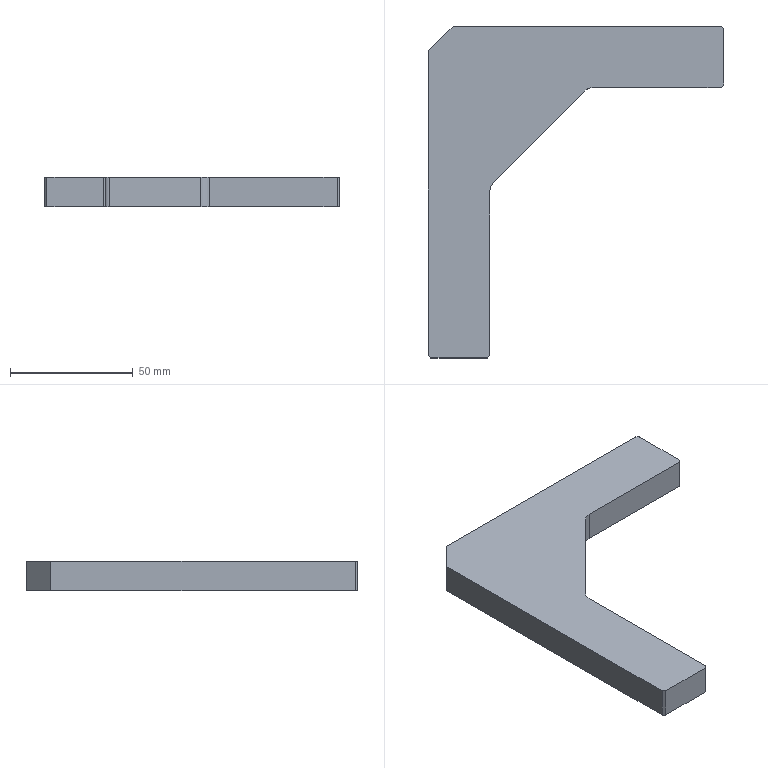Part | SolidWorks | features BaseBody 1 | 1 solid | 16 faces | box 120 x 135 x 12 mm | volume 77989 mm3 | plane 14 | cylinder 2 | commonest cylinder face diameters 10 x2
STEP:
#1=CARTESIAN_POINT('',(120.,-1.,12.));
#2=VERTEX_POINT('',#1);
#3=CARTESIAN_POINT('',(119.,0.,12.));
#4=VERTEX_POINT('',#3);
#5=CARTESIAN_POINT('',(119.,0.,12.));
#6=DIRECTION('',(-0.7071,0.7071,0.));
#7=VECTOR('',#6,1000.);
#8=LINE('',#5,#7);
#9=EDGE_CURVE('',#2,#4,#8,.T.);
#10=ORIENTED_EDGE('',*,*,#9,.F.);
#11=CARTESIAN_POINT('',(120.,-1.,0.));
#12=VERTEX_POINT('',#11);
#13=CARTESIAN_POINT('',(120.,-1.,12.));
#14=DIRECTION('',(0.,0.,1.));
#15=VECTOR('',#14,1000.);
#16=LINE('',#13,#15);
#17=EDGE_CURVE('',#12,#2,#16,.T.);
#18=ORIENTED_EDGE('',*,*,#17,.F.);
#19=CARTESIAN_POINT('',(119.,0.,0.));
#20=VERTEX_POINT('',#19);
#21=CARTESIAN_POINT('',(59.5,59.5,0.));
#22=DIRECTION('',(0.7071,-0.7071,0.));
#23=VECTOR('',#22,1000.);
#24=LINE('',#21,#23);
#25=EDGE_CURVE('',#20,#12,#24,.T.);
#26=ORIENTED_EDGE('',*,*,#25,.F.);
#27=CARTESIAN_POINT('',(119.,0.,12.));
#28=DIRECTION('',(0.,0.,-1.));
#29=VECTOR('',#28,1000.);
#30=LINE('',#27,#29);
#31=EDGE_CURVE('',#4,#20,#30,.T.);
#32=ORIENTED_EDGE('',*,*,#31,.F.);
#33=EDGE_LOOP('',(#10,#18,#26,#32));
#34=FACE_OUTER_BOUND('',#33,.T.);
#35=CARTESIAN_POINT('',(119.,0.,12.));
#36=DIRECTION('',(-0.7071,-0.7071,0.));
#37=DIRECTION('',(-0.7071,0.7071,0.));
#38=AXIS2_PLACEMENT_3D('',#35,#36,#37);
#39=PLANE('',#38);
#40=ADVANCED_FACE('',(#34),#39,.F.);
#41=CARTESIAN_POINT('',(119.,-25.,12.));
#42=VERTEX_POINT('',#41);
#43=CARTESIAN_POINT('',(120.,-24.,12.));
#44=VERTEX_POINT('',#43);
#45=CARTESIAN_POINT('',(120.,-24.,12.));
#46=DIRECTION('',(0.7071,0.7071,0.));
#47=VECTOR('',#46,1000.);
#48=LINE('',#45,#47);
#49=EDGE_CURVE('',#42,#44,#48,.T.);
#50=ORIENTED_EDGE('',*,*,#49,.F.);
#51=CARTESIAN_POINT('',(119.,-25.,0.));
#52=VERTEX_POINT('',#51);
#53=CARTESIAN_POINT('',(119.,-25.,12.));
#54=DIRECTION('',(0.,0.,1.));
#55=VECTOR('',#54,1000.);
#56=LINE('',#53,#55);
#57=EDGE_CURVE('',#52,#42,#56,.T.);
#58=ORIENTED_EDGE('',*,*,#57,.F.);
#59=CARTESIAN_POINT('',(120.,-24.,0.));
#60=VERTEX_POINT('',#59);
#61=CARTESIAN_POINT('',(72.,-72.,0.));
#62=DIRECTION('',(-0.7071,-0.7071,0.));
#63=VECTOR('',#62,1000.);
#64=LINE('',#61,#63);
#65=EDGE_CURVE('',#60,#52,#64,.T.);
#66=ORIENTED_EDGE('',*,*,#65,.F.);
#67=CARTESIAN_POINT('',(120.,-24.,12.));
#68=DIRECTION('',(0.,0.,-1.));
#69=VECTOR('',#68,1000.);
#70=LINE('',#67,#69);
#71=EDGE_CURVE('',#44,#60,#70,.T.);
#72=ORIENTED_EDGE('',*,*,#71,.F.);
#73=EDGE_LOOP('',(#50,#58,#66,#72));
#74=FACE_OUTER_BOUND('',#73,.T.);
#75=CARTESIAN_POINT('',(120.,-24.,12.));
#76=DIRECTION('',(-0.7071,0.7071,0.));
#77=DIRECTION('',(0.,0.,1.));
#78=AXIS2_PLACEMENT_3D('',#75,#76,#77);
#79=PLANE('',#78);
#80=ADVANCED_FACE('',(#74),#79,.F.);
#81=CARTESIAN_POINT('',(24.,-135.,12.));
#82=VERTEX_POINT('',#81);
#83=CARTESIAN_POINT('',(25.,-134.,12.));
#84=VERTEX_POINT('',#83);
#85=CARTESIAN_POINT('',(25.,-134.,12.));
#86=DIRECTION('',(0.7071,0.7071,0.));
#87=VECTOR('',#86,1000.);
#88=LINE('',#85,#87);
#89=EDGE_CURVE('',#82,#84,#88,.T.);
#90=ORIENTED_EDGE('',*,*,#89,.F.);
#91=CARTESIAN_POINT('',(24.,-135.,0.));
#92=VERTEX_POINT('',#91);
#93=CARTESIAN_POINT('',(24.,-135.,12.));
#94=DIRECTION('',(0.,0.,1.));
#95=VECTOR('',#94,1000.);
#96=LINE('',#93,#95);
#97=EDGE_CURVE('',#92,#82,#96,.T.);
#98=ORIENTED_EDGE('',*,*,#97,.F.);
#99=CARTESIAN_POINT('',(25.,-134.,0.));
#100=VERTEX_POINT('',#99);
#101=CARTESIAN_POINT('',(79.5,-79.5,0.));
#102=DIRECTION('',(-0.7071,-0.7071,0.));
#103=VECTOR('',#102,1000.);
#104=LINE('',#101,#103);
#105=EDGE_CURVE('',#100,#92,#104,.T.);
#106=ORIENTED_EDGE('',*,*,#105,.F.);
#107=CARTESIAN_POINT('',(25.,-134.,12.));
#108=DIRECTION('',(0.,0.,-1.));
#109=VECTOR('',#108,1000.);
#110=LINE('',#107,#109);
#111=EDGE_CURVE('',#84,#100,#110,.T.);
#112=ORIENTED_EDGE('',*,*,#111,.F.);
#113=EDGE_LOOP('',(#90,#98,#106,#112));
#114=FACE_OUTER_BOUND('',#113,.T.);
#115=CARTESIAN_POINT('',(25.,-134.,12.));
#116=DIRECTION('',(-0.7071,0.7071,0.));
#117=DIRECTION('',(0.,0.,1.));
#118=AXIS2_PLACEMENT_3D('',#115,#116,#117);
#119=PLANE('',#118);
#120=ADVANCED_FACE('',(#114),#119,.F.);
#121=CARTESIAN_POINT('',(0.,-134.,12.));
#122=VERTEX_POINT('',#121);
#123=CARTESIAN_POINT('',(1.,-135.,12.));
#124=VERTEX_POINT('',#123);
#125=CARTESIAN_POINT('',(1.,-135.,12.));
#126=DIRECTION('',(0.7071,-0.7071,0.));
#127=VECTOR('',#126,1000.);
#128=LINE('',#125,#127);
#129=EDGE_CURVE('',#122,#124,#128,.T.);
#130=ORIENTED_EDGE('',*,*,#129,.F.);
#131=CARTESIAN_POINT('',(0.,-134.,0.));
#132=VERTEX_POINT('',#131);
#133=CARTESIAN_POINT('',(0.,-134.,12.));
#134=DIRECTION('',(0.,0.,1.));
#135=VECTOR('',#134,1000.);
#136=LINE('',#133,#135);
#137=EDGE_CURVE('',#132,#122,#136,.T.);
#138=ORIENTED_EDGE('',*,*,#137,.F.);
#139=CARTESIAN_POINT('',(1.,-135.,0.));
#140=VERTEX_POINT('',#139);
#141=CARTESIAN_POINT('',(-67.,-67.,0.));
#142=DIRECTION('',(-0.7071,0.7071,0.));
#143=VECTOR('',#142,1000.);
#144=LINE('',#141,#143);
#145=EDGE_CURVE('',#140,#132,#144,.T.);
#146=ORIENTED_EDGE('',*,*,#145,.F.);
#147=CARTESIAN_POINT('',(1.,-135.,12.));
#148=DIRECTION('',(0.,0.,-1.));
#149=VECTOR('',#148,1000.);
#150=LINE('',#147,#149);
#151=EDGE_CURVE('',#124,#140,#150,.T.);
#152=ORIENTED_EDGE('',*,*,#151,.F.);
#153=EDGE_LOOP('',(#130,#138,#146,#152));
#154=FACE_OUTER_BOUND('',#153,.T.);
#155=CARTESIAN_POINT('',(1.,-135.,12.));
#156=DIRECTION('',(0.7071,0.7071,0.));
#157=DIRECTION('',(0.,0.,-1.));
#158=AXIS2_PLACEMENT_3D('',#155,#156,#157);
#159=PLANE('',#158);
#160=ADVANCED_FACE('',(#154),#159,.F.);
#161=CARTESIAN_POINT('',(25.,-67.071,12.));
#162=VERTEX_POINT('',#161);
#163=CARTESIAN_POINT('',(26.464,-63.536,12.));
#164=VERTEX_POINT('',#163);
#165=CARTESIAN_POINT('',(30.,-67.071,12.));
#166=DIRECTION('',(0.,0.,-1.));
#167=DIRECTION('',(-1.,0.,0.));
#168=AXIS2_PLACEMENT_3D('',#165,#166,#167);
#169=CIRCLE('',#168,5.);
#170=EDGE_CURVE('',#162,#164,#169,.T.);
#171=ORIENTED_EDGE('',*,*,#170,.F.);
#172=CARTESIAN_POINT('',(25.,-67.071,0.));
#173=VERTEX_POINT('',#172);
#174=CARTESIAN_POINT('',(25.,-67.071,12.));
#175=DIRECTION('',(0.,0.,1.));
#176=VECTOR('',#175,1000.);
#177=LINE('',#174,#176);
#178=EDGE_CURVE('',#173,#162,#177,.T.);
#179=ORIENTED_EDGE('',*,*,#178,.F.);
#180=CARTESIAN_POINT('',(26.464,-63.536,0.));
#181=VERTEX_POINT('',#180);
#182=CARTESIAN_POINT('',(30.,-67.071,0.));
#183=DIRECTION('',(0.,0.,1.));
#184=DIRECTION('',(-1.,0.,0.));
#185=AXIS2_PLACEMENT_3D('',#182,#183,#184);
#186=CIRCLE('',#185,5.);
#187=EDGE_CURVE('',#181,#173,#186,.T.);
#188=ORIENTED_EDGE('',*,*,#187,.F.);
#189=CARTESIAN_POINT('',(26.464,-63.536,0.));
#190=DIRECTION('',(0.,0.,-1.));
#191=VECTOR('',#190,1000.);
#192=LINE('',#189,#191);
#193=EDGE_CURVE('',#164,#181,#192,.T.);
#194=ORIENTED_EDGE('',*,*,#193,.F.);
#195=EDGE_LOOP('',(#171,#179,#188,#194));
#196=FACE_OUTER_BOUND('',#195,.T.);
#197=CARTESIAN_POINT('',(30.,-67.071,12.));
#198=DIRECTION('',(0.,0.,1.));
#199=DIRECTION('',(1.,0.,0.));
#200=AXIS2_PLACEMENT_3D('',#197,#198,#199);
#201=CYLINDRICAL_SURFACE('',#200,5.);
#202=ADVANCED_FACE('',(#196),#201,.F.);
#203=CARTESIAN_POINT('',(63.536,-26.464,12.));
#204=VERTEX_POINT('',#203);
#205=CARTESIAN_POINT('',(67.071,-25.,12.));
#206=VERTEX_POINT('',#205);
#207=CARTESIAN_POINT('',(67.071,-30.,12.));
#208=DIRECTION('',(0.,0.,-1.));
#209=DIRECTION('',(-1.,0.,0.));
#210=AXIS2_PLACEMENT_3D('',#207,#208,#209);
#211=CIRCLE('',#210,5.);
#212=EDGE_CURVE('',#204,#206,#211,.T.);
#213=ORIENTED_EDGE('',*,*,#212,.F.);
#214=CARTESIAN_POINT('',(63.536,-26.464,0.));
#215=VERTEX_POINT('',#214);
#216=CARTESIAN_POINT('',(63.536,-26.464,12.));
#217=DIRECTION('',(0.,0.,1.));
#218=VECTOR('',#217,1000.);
#219=LINE('',#216,#218);
#220=EDGE_CURVE('',#215,#204,#219,.T.);
#221=ORIENTED_EDGE('',*,*,#220,.F.);
#222=CARTESIAN_POINT('',(67.071,-25.,0.));
#223=VERTEX_POINT('',#222);
#224=CARTESIAN_POINT('',(67.071,-30.,0.));
#225=DIRECTION('',(0.,0.,1.));
#226=DIRECTION('',(-1.,0.,0.));
#227=AXIS2_PLACEMENT_3D('',#224,#225,#226);
#228=CIRCLE('',#227,5.);
#229=EDGE_CURVE('',#223,#215,#228,.T.);
#230=ORIENTED_EDGE('',*,*,#229,.F.);
#231=CARTESIAN_POINT('',(67.071,-25.,0.));
#232=DIRECTION('',(0.,0.,-1.));
#233=VECTOR('',#232,1000.);
#234=LINE('',#231,#233);
#235=EDGE_CURVE('',#206,#223,#234,.T.);
#236=ORIENTED_EDGE('',*,*,#235,.F.);
#237=EDGE_LOOP('',(#213,#221,#230,#236));
#238=FACE_OUTER_BOUND('',#237,.T.);
#239=CARTESIAN_POINT('',(67.071,-30.,12.));
#240=DIRECTION('',(0.,0.,1.));
#241=DIRECTION('',(1.,0.,0.));
#242=AXIS2_PLACEMENT_3D('',#239,#240,#241);
#243=CYLINDRICAL_SURFACE('',#242,5.);
#244=ADVANCED_FACE('',(#238),#243,.F.);
#245=CARTESIAN_POINT('',(10.,0.,12.));
#246=VERTEX_POINT('',#245);
#247=CARTESIAN_POINT('',(0.,-10.,12.));
#248=VERTEX_POINT('',#247);
#249=CARTESIAN_POINT('',(0.,-10.,12.));
#250=DIRECTION('',(-0.7071,-0.7071,0.));
#251=VECTOR('',#250,1000.);
#252=LINE('',#249,#251);
#253=EDGE_CURVE('',#246,#248,#252,.T.);
#254=ORIENTED_EDGE('',*,*,#253,.F.);
#255=CARTESIAN_POINT('',(10.,0.,0.));
#256=VERTEX_POINT('',#255);
#257=CARTESIAN_POINT('',(10.,0.,12.));
#258=DIRECTION('',(0.,0.,1.));
#259=VECTOR('',#258,1000.);
#260=LINE('',#257,#259);
#261=EDGE_CURVE('',#256,#246,#260,.T.);
#262=ORIENTED_EDGE('',*,*,#261,.F.);
#263=CARTESIAN_POINT('',(0.,-10.,0.));
#264=VERTEX_POINT('',#263);
#265=CARTESIAN_POINT('',(5.,-5.,0.));
#266=DIRECTION('',(0.7071,0.7071,0.));
#267=VECTOR('',#266,1000.);
#268=LINE('',#265,#267);
#269=EDGE_CURVE('',#264,#256,#268,.T.);
#270=ORIENTED_EDGE('',*,*,#269,.F.);
#271=CARTESIAN_POINT('',(0.,-10.,12.));
#272=DIRECTION('',(0.,0.,-1.));
#273=VECTOR('',#272,1000.);
#274=LINE('',#271,#273);
#275=EDGE_CURVE('',#248,#264,#274,.T.);
#276=ORIENTED_EDGE('',*,*,#275,.F.);
#277=EDGE_LOOP('',(#254,#262,#270,#276));
#278=FACE_OUTER_BOUND('',#277,.T.);
#279=CARTESIAN_POINT('',(0.,-10.,12.));
#280=DIRECTION('',(0.7071,-0.7071,0.));
#281=DIRECTION('',(0.,0.,-1.));
#282=AXIS2_PLACEMENT_3D('',#279,#280,#281);
#283=PLANE('',#282);
#284=ADVANCED_FACE('',(#278),#283,.F.);
#285=CARTESIAN_POINT('',(25.,-135.,0.));
#286=DIRECTION('',(1.,0.,0.));
#287=VECTOR('',#286,1000.);
#288=LINE('',#285,#287);
#289=EDGE_CURVE('',#140,#92,#288,.T.);
#290=ORIENTED_EDGE('',*,*,#289,.F.);
#291=ORIENTED_EDGE('',*,*,#145,.T.);
#292=CARTESIAN_POINT('',(0.,-135.,0.));
#293=DIRECTION('',(0.,-1.,0.));
#294=VECTOR('',#293,1000.);
#295=LINE('',#292,#294);
#296=EDGE_CURVE('',#264,#132,#295,.T.);
#297=ORIENTED_EDGE('',*,*,#296,.F.);
#298=ORIENTED_EDGE('',*,*,#269,.T.);
#299=CARTESIAN_POINT('',(0.,0.,0.));
#300=DIRECTION('',(-1.,0.,0.));
#301=VECTOR('',#300,1000.);
#302=LINE('',#299,#301);
#303=EDGE_CURVE('',#20,#256,#302,.T.);
#304=ORIENTED_EDGE('',*,*,#303,.F.);
#305=ORIENTED_EDGE('',*,*,#25,.T.);
#306=CARTESIAN_POINT('',(120.,0.,0.));
#307=DIRECTION('',(0.,1.,0.));
#308=VECTOR('',#307,1000.);
#309=LINE('',#306,#308);
#310=EDGE_CURVE('',#60,#12,#309,.T.);
#311=ORIENTED_EDGE('',*,*,#310,.F.);
#312=ORIENTED_EDGE('',*,*,#65,.T.);
#313=CARTESIAN_POINT('',(120.,-25.,0.));
#314=DIRECTION('',(1.,0.,0.));
#315=VECTOR('',#314,1000.);
#316=LINE('',#313,#315);
#317=EDGE_CURVE('',#223,#52,#316,.T.);
#318=ORIENTED_EDGE('',*,*,#317,.F.);
#319=ORIENTED_EDGE('',*,*,#229,.T.);
#320=CARTESIAN_POINT('',(65.,-25.,0.));
#321=DIRECTION('',(0.7071,0.7071,0.));
#322=VECTOR('',#321,1000.);
#323=LINE('',#320,#322);
#324=EDGE_CURVE('',#181,#215,#323,.T.);
#325=ORIENTED_EDGE('',*,*,#324,.F.);
#326=ORIENTED_EDGE('',*,*,#187,.T.);
#327=CARTESIAN_POINT('',(25.,-65.,0.));
#328=DIRECTION('',(0.,1.,0.));
#329=VECTOR('',#328,1000.);
#330=LINE('',#327,#329);
#331=EDGE_CURVE('',#100,#173,#330,.T.);
#332=ORIENTED_EDGE('',*,*,#331,.F.);
#333=ORIENTED_EDGE('',*,*,#105,.T.);
#334=EDGE_LOOP('',(#290,#291,#297,#298,#304,#305,#311,#312,#318,#319,#325,#326,#332,#333));
#335=FACE_OUTER_BOUND('',#334,.T.);
#336=CARTESIAN_POINT('',(0.,0.,0.));
#337=DIRECTION('',(0.,0.,-1.));
#338=DIRECTION('',(0.,-1.,0.));
#339=AXIS2_PLACEMENT_3D('',#336,#337,#338);
#340=PLANE('',#339);
#341=ADVANCED_FACE('',(#335),#340,.T.);
#342=CARTESIAN_POINT('',(0.,-135.,12.));
#343=DIRECTION('',(0.,-1.,0.));
#344=VECTOR('',#343,1000.);
#345=LINE('',#342,#344);
#346=EDGE_CURVE('',#248,#122,#345,.T.);
#347=ORIENTED_EDGE('',*,*,#346,.T.);
#348=ORIENTED_EDGE('',*,*,#129,.T.);
#349=CARTESIAN_POINT('',(25.,-135.,12.));
#350=DIRECTION('',(1.,0.,0.));
#351=VECTOR('',#350,1000.);
#352=LINE('',#349,#351);
#353=EDGE_CURVE('',#124,#82,#352,.T.);
#354=ORIENTED_EDGE('',*,*,#353,.T.);
#355=ORIENTED_EDGE('',*,*,#89,.T.);
#356=CARTESIAN_POINT('',(25.,-65.,12.));
#357=DIRECTION('',(0.,1.,0.));
#358=VECTOR('',#357,1000.);
#359=LINE('',#356,#358);
#360=EDGE_CURVE('',#84,#162,#359,.T.);
#361=ORIENTED_EDGE('',*,*,#360,.T.);
#362=ORIENTED_EDGE('',*,*,#170,.T.);
#363=CARTESIAN_POINT('',(65.,-25.,12.));
#364=DIRECTION('',(0.7071,0.7071,0.));
#365=VECTOR('',#364,1000.);
#366=LINE('',#363,#365);
#367=EDGE_CURVE('',#164,#204,#366,.T.);
#368=ORIENTED_EDGE('',*,*,#367,.T.);
#369=ORIENTED_EDGE('',*,*,#212,.T.);
#370=CARTESIAN_POINT('',(120.,-25.,12.));
#371=DIRECTION('',(1.,0.,0.));
#372=VECTOR('',#371,1000.);
#373=LINE('',#370,#372);
#374=EDGE_CURVE('',#206,#42,#373,.T.);
#375=ORIENTED_EDGE('',*,*,#374,.T.);
#376=ORIENTED_EDGE('',*,*,#49,.T.);
#377=CARTESIAN_POINT('',(120.,0.,12.));
#378=DIRECTION('',(0.,1.,0.));
#379=VECTOR('',#378,1000.);
#380=LINE('',#377,#379);
#381=EDGE_CURVE('',#44,#2,#380,.T.);
#382=ORIENTED_EDGE('',*,*,#381,.T.);
#383=ORIENTED_EDGE('',*,*,#9,.T.);
#384=CARTESIAN_POINT('',(0.,0.,12.));
#385=DIRECTION('',(-1.,0.,0.));
#386=VECTOR('',#385,1000.);
#387=LINE('',#384,#386);
#388=EDGE_CURVE('',#4,#246,#387,.T.);
#389=ORIENTED_EDGE('',*,*,#388,.T.);
#390=ORIENTED_EDGE('',*,*,#253,.T.);
#391=EDGE_LOOP('',(#347,#348,#354,#355,#361,#362,#368,#369,#375,#376,#382,#383,#389,#390));
#392=FACE_OUTER_BOUND('',#391,.T.);
#393=CARTESIAN_POINT('',(0.,0.,12.));
#394=DIRECTION('',(0.,0.,-1.));
#395=DIRECTION('',(0.,-1.,0.));
#396=AXIS2_PLACEMENT_3D('',#393,#394,#395);
#397=PLANE('',#396);
#398=ADVANCED_FACE('',(#392),#397,.F.);
#399=ORIENTED_EDGE('',*,*,#388,.F.);
#400=ORIENTED_EDGE('',*,*,#31,.T.);
#401=ORIENTED_EDGE('',*,*,#303,.T.);
#402=ORIENTED_EDGE('',*,*,#261,.T.);
#403=EDGE_LOOP('',(#399,#400,#401,#402));
#404=FACE_OUTER_BOUND('',#403,.T.);
#405=CARTESIAN_POINT('',(0.,0.,12.));
#406=DIRECTION('',(0.,-1.,0.));
#407=DIRECTION('',(0.,0.,-1.));
#408=AXIS2_PLACEMENT_3D('',#405,#406,#407);
#409=PLANE('',#408);
#410=ADVANCED_FACE('',(#404),#409,.F.);
#411=ORIENTED_EDGE('',*,*,#381,.F.);
#412=ORIENTED_EDGE('',*,*,#71,.T.);
#413=ORIENTED_EDGE('',*,*,#310,.T.);
#414=ORIENTED_EDGE('',*,*,#17,.T.);
#415=EDGE_LOOP('',(#411,#412,#413,#414));
#416=FACE_OUTER_BOUND('',#415,.T.);
#417=CARTESIAN_POINT('',(120.,0.,12.));
#418=DIRECTION('',(-1.,0.,0.));
#419=DIRECTION('',(0.,0.,1.));
#420=AXIS2_PLACEMENT_3D('',#417,#418,#419);
#421=PLANE('',#420);
#422=ADVANCED_FACE('',(#416),#421,.F.);
#423=ORIENTED_EDGE('',*,*,#317,.T.);
#424=ORIENTED_EDGE('',*,*,#57,.T.);
#425=ORIENTED_EDGE('',*,*,#374,.F.);
#426=ORIENTED_EDGE('',*,*,#235,.T.);
#427=EDGE_LOOP('',(#423,#424,#425,#426));
#428=FACE_OUTER_BOUND('',#427,.T.);
#429=CARTESIAN_POINT('',(120.,-25.,12.));
#430=DIRECTION('',(0.,1.,0.));
#431=DIRECTION('',(1.,0.,0.));
#432=AXIS2_PLACEMENT_3D('',#429,#430,#431);
#433=PLANE('',#432);
#434=ADVANCED_FACE('',(#428),#433,.F.);
#435=ORIENTED_EDGE('',*,*,#324,.T.);
#436=ORIENTED_EDGE('',*,*,#220,.T.);
#437=ORIENTED_EDGE('',*,*,#367,.F.);
#438=ORIENTED_EDGE('',*,*,#193,.T.);
#439=EDGE_LOOP('',(#435,#436,#437,#438));
#440=FACE_OUTER_BOUND('',#439,.T.);
#441=CARTESIAN_POINT('',(65.,-25.,12.));
#442=DIRECTION('',(-0.7071,0.7071,0.));
#443=DIRECTION('',(0.,0.,1.));
#444=AXIS2_PLACEMENT_3D('',#441,#442,#443);
#445=PLANE('',#444);
#446=ADVANCED_FACE('',(#440),#445,.F.);
#447=ORIENTED_EDGE('',*,*,#360,.F.);
#448=ORIENTED_EDGE('',*,*,#111,.T.);
#449=ORIENTED_EDGE('',*,*,#331,.T.);
#450=ORIENTED_EDGE('',*,*,#178,.T.);
#451=EDGE_LOOP('',(#447,#448,#449,#450));
#452=FACE_OUTER_BOUND('',#451,.T.);
#453=CARTESIAN_POINT('',(25.,-65.,12.));
#454=DIRECTION('',(-1.,0.,0.));
#455=DIRECTION('',(0.,1.,0.));
#456=AXIS2_PLACEMENT_3D('',#453,#454,#455);
#457=PLANE('',#456);
#458=ADVANCED_FACE('',(#452),#457,.F.);
#459=ORIENTED_EDGE('',*,*,#353,.F.);
#460=ORIENTED_EDGE('',*,*,#151,.T.);
#461=ORIENTED_EDGE('',*,*,#289,.T.);
#462=ORIENTED_EDGE('',*,*,#97,.T.);
#463=EDGE_LOOP('',(#459,#460,#461,#462));
#464=FACE_OUTER_BOUND('',#463,.T.);
#465=CARTESIAN_POINT('',(25.,-135.,12.));
#466=DIRECTION('',(0.,1.,0.));
#467=DIRECTION('',(1.,0.,0.));
#468=AXIS2_PLACEMENT_3D('',#465,#466,#467);
#469=PLANE('',#468);
#470=ADVANCED_FACE('',(#464),#469,.F.);
#471=ORIENTED_EDGE('',*,*,#296,.T.);
#472=ORIENTED_EDGE('',*,*,#137,.T.);
#473=ORIENTED_EDGE('',*,*,#346,.F.);
#474=ORIENTED_EDGE('',*,*,#275,.T.);
#475=EDGE_LOOP('',(#471,#472,#473,#474));
#476=FACE_OUTER_BOUND('',#475,.T.);
#477=CARTESIAN_POINT('',(0.,-135.,12.));
#478=DIRECTION('',(1.,0.,0.));
#479=DIRECTION('',(0.,1.,0.));
#480=AXIS2_PLACEMENT_3D('',#477,#478,#479);
#481=PLANE('',#480);
#482=ADVANCED_FACE('',(#476),#481,.F.);
#483=CLOSED_SHELL('',(#40,#80,#120,#160,#202,#244,#284,#341,#398,#410,#422,#434,#446,#458,#470,#482));
#484=MANIFOLD_SOLID_BREP('',#483);
#485=CARTESIAN_POINT('',(0.,0.,0.));
#486=DIRECTION('',(0.,0.,1.));
#487=DIRECTION('',(1.,0.,0.));
#488=AXIS2_PLACEMENT_3D('',#485,#486,#487);
#489=(LENGTH_UNIT()NAMED_UNIT(*)SI_UNIT(.MILLI.,.METRE.));
#490=UNCERTAINTY_MEASURE_WITH_UNIT(LENGTH_MEASURE(0.00001),#489,'','');
#491=(NAMED_UNIT(*)PLANE_ANGLE_UNIT()SI_UNIT($,.RADIAN.));
#492=(NAMED_UNIT(*)SI_UNIT($,.STERADIAN.)SOLID_ANGLE_UNIT());
#493=(GEOMETRIC_REPRESENTATION_CONTEXT(3)GLOBAL_UNCERTAINTY_ASSIGNED_CONTEXT((#490))GLOBAL_UNIT_ASSIGNED_CONTEXT((#489,#491,#492))REPRESENTATION_CONTEXT('',''));
#494=ADVANCED_BREP_SHAPE_REPRESENTATION('',(#484,#488),#493);